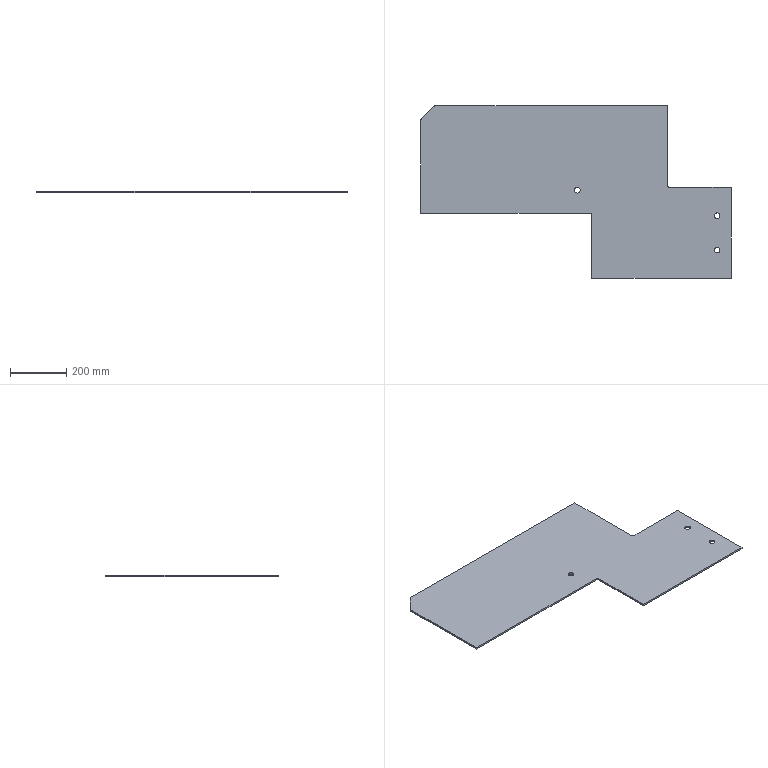Part | SolidWorks | features Fillet 1, FlatPattern 1, SMBaseFlange 1, SheetMetal 1 | 1 solid | 21 faces | box 1100 x 612 x 6 mm | volume 2796793 mm3 | plane 11 | cylinder 10 | commonest cylinder face diameters 20 x8 12 x2
STEP:
#1=CARTESIAN_POINT('',(-555.,312.,-6.));
#2=VERTEX_POINT('',#1);
#3=CARTESIAN_POINT('',(-535.,312.,-6.));
#4=VERTEX_POINT('',#3);
#5=CARTESIAN_POINT('',(-545.,312.,-6.));
#6=DIRECTION('',(0.,0.,1.));
#7=DIRECTION('',(1.,0.,0.));
#8=AXIS2_PLACEMENT_3D('',#5,#6,#7);
#9=CIRCLE('',#8,10.);
#10=EDGE_CURVE('',#2,#4,#9,.T.);
#11=ORIENTED_EDGE('',*,*,#10,.F.);
#12=CARTESIAN_POINT('',(-555.,312.,0.));
#13=VERTEX_POINT('',#12);
#14=CARTESIAN_POINT('',(-555.,312.,-6.));
#15=DIRECTION('',(0.,0.,1.));
#16=VECTOR('',#15,1000.);
#17=LINE('',#14,#16);
#18=EDGE_CURVE('',#2,#13,#17,.T.);
#19=ORIENTED_EDGE('',*,*,#18,.T.);
#20=CARTESIAN_POINT('',(-535.,312.,0.));
#21=VERTEX_POINT('',#20);
#22=CARTESIAN_POINT('',(-545.,312.,0.));
#23=DIRECTION('',(0.,0.,1.));
#24=DIRECTION('',(1.,0.,0.));
#25=AXIS2_PLACEMENT_3D('',#22,#23,#24);
#26=CIRCLE('',#25,10.);
#27=EDGE_CURVE('',#13,#21,#26,.T.);
#28=ORIENTED_EDGE('',*,*,#27,.T.);
#29=CARTESIAN_POINT('',(-535.,312.,-6.));
#30=DIRECTION('',(0.,0.,1.));
#31=VECTOR('',#30,1000.);
#32=LINE('',#29,#31);
#33=EDGE_CURVE('',#4,#21,#32,.T.);
#34=ORIENTED_EDGE('',*,*,#33,.F.);
#35=EDGE_LOOP('',(#11,#19,#28,#34));
#36=FACE_OUTER_BOUND('',#35,.T.);
#37=CARTESIAN_POINT('',(-545.,312.,-6.));
#38=DIRECTION('',(0.,0.,1.));
#39=DIRECTION('',(1.,0.,0.));
#40=AXIS2_PLACEMENT_3D('',#37,#38,#39);
#41=CYLINDRICAL_SURFACE('',#40,10.);
#42=ADVANCED_FACE('',(#36),#41,.F.);
#43=CARTESIAN_POINT('',(-60.,222.,-6.));
#44=VERTEX_POINT('',#43);
#45=CARTESIAN_POINT('',(-40.,222.,-6.));
#46=VERTEX_POINT('',#45);
#47=CARTESIAN_POINT('',(-50.,222.,-6.));
#48=DIRECTION('',(0.,0.,1.));
#49=DIRECTION('',(1.,0.,0.));
#50=AXIS2_PLACEMENT_3D('',#47,#48,#49);
#51=CIRCLE('',#50,10.);
#52=EDGE_CURVE('',#44,#46,#51,.T.);
#53=ORIENTED_EDGE('',*,*,#52,.F.);
#54=CARTESIAN_POINT('',(-60.,222.,0.));
#55=VERTEX_POINT('',#54);
#56=CARTESIAN_POINT('',(-60.,222.,-6.));
#57=DIRECTION('',(0.,0.,1.));
#58=VECTOR('',#57,1000.);
#59=LINE('',#56,#58);
#60=EDGE_CURVE('',#44,#55,#59,.T.);
#61=ORIENTED_EDGE('',*,*,#60,.T.);
#62=CARTESIAN_POINT('',(-40.,222.,0.));
#63=VERTEX_POINT('',#62);
#64=CARTESIAN_POINT('',(-50.,222.,0.));
#65=DIRECTION('',(0.,0.,1.));
#66=DIRECTION('',(1.,0.,0.));
#67=AXIS2_PLACEMENT_3D('',#64,#65,#66);
#68=CIRCLE('',#67,10.);
#69=EDGE_CURVE('',#55,#63,#68,.T.);
#70=ORIENTED_EDGE('',*,*,#69,.T.);
#71=CARTESIAN_POINT('',(-40.,222.,-6.));
#72=DIRECTION('',(0.,0.,1.));
#73=VECTOR('',#72,1000.);
#74=LINE('',#71,#73);
#75=EDGE_CURVE('',#46,#63,#74,.T.);
#76=ORIENTED_EDGE('',*,*,#75,.F.);
#77=EDGE_LOOP('',(#53,#61,#70,#76));
#78=FACE_OUTER_BOUND('',#77,.T.);
#79=CARTESIAN_POINT('',(-50.,222.,-6.));
#80=DIRECTION('',(0.,0.,1.));
#81=DIRECTION('',(1.,0.,0.));
#82=AXIS2_PLACEMENT_3D('',#79,#80,#81);
#83=CYLINDRICAL_SURFACE('',#82,10.);
#84=ADVANCED_FACE('',(#78),#83,.F.);
#85=CARTESIAN_POINT('',(-60.,100.,-6.));
#86=VERTEX_POINT('',#85);
#87=CARTESIAN_POINT('',(-40.,100.,-6.));
#88=VERTEX_POINT('',#87);
#89=CARTESIAN_POINT('',(-50.,100.,-6.));
#90=DIRECTION('',(0.,0.,1.));
#91=DIRECTION('',(1.,0.,0.));
#92=AXIS2_PLACEMENT_3D('',#89,#90,#91);
#93=CIRCLE('',#92,10.);
#94=EDGE_CURVE('',#86,#88,#93,.T.);
#95=ORIENTED_EDGE('',*,*,#94,.F.);
#96=CARTESIAN_POINT('',(-60.,100.,0.));
#97=VERTEX_POINT('',#96);
#98=CARTESIAN_POINT('',(-60.,100.,-6.));
#99=DIRECTION('',(0.,0.,1.));
#100=VECTOR('',#99,1000.);
#101=LINE('',#98,#100);
#102=EDGE_CURVE('',#86,#97,#101,.T.);
#103=ORIENTED_EDGE('',*,*,#102,.T.);
#104=CARTESIAN_POINT('',(-40.,100.,0.));
#105=VERTEX_POINT('',#104);
#106=CARTESIAN_POINT('',(-50.,100.,0.));
#107=DIRECTION('',(0.,0.,1.));
#108=DIRECTION('',(1.,0.,0.));
#109=AXIS2_PLACEMENT_3D('',#106,#107,#108);
#110=CIRCLE('',#109,10.);
#111=EDGE_CURVE('',#97,#105,#110,.T.);
#112=ORIENTED_EDGE('',*,*,#111,.T.);
#113=CARTESIAN_POINT('',(-40.,100.,-6.));
#114=DIRECTION('',(0.,0.,1.));
#115=VECTOR('',#114,1000.);
#116=LINE('',#113,#115);
#117=EDGE_CURVE('',#88,#105,#116,.T.);
#118=ORIENTED_EDGE('',*,*,#117,.F.);
#119=EDGE_LOOP('',(#95,#103,#112,#118));
#120=FACE_OUTER_BOUND('',#119,.T.);
#121=CARTESIAN_POINT('',(-50.,100.,-6.));
#122=DIRECTION('',(0.,0.,1.));
#123=DIRECTION('',(1.,0.,0.));
#124=AXIS2_PLACEMENT_3D('',#121,#122,#123);
#125=CYLINDRICAL_SURFACE('',#124,10.);
#126=ADVANCED_FACE('',(#120),#125,.F.);
#127=CARTESIAN_POINT('',(0.,0.,0.));
#128=VERTEX_POINT('',#127);
#129=CARTESIAN_POINT('',(0.,322.,0.));
#130=VERTEX_POINT('',#129);
#131=CARTESIAN_POINT('',(0.,322.,0.));
#132=DIRECTION('',(0.,1.,0.));
#133=VECTOR('',#132,1000.);
#134=LINE('',#131,#133);
#135=EDGE_CURVE('',#128,#130,#134,.T.);
#136=ORIENTED_EDGE('',*,*,#135,.F.);
#137=CARTESIAN_POINT('',(0.,0.,-6.));
#138=VERTEX_POINT('',#137);
#139=CARTESIAN_POINT('',(0.,0.,-6.));
#140=DIRECTION('',(0.,0.,1.));
#141=VECTOR('',#140,1000.);
#142=LINE('',#139,#141);
#143=EDGE_CURVE('',#138,#128,#142,.T.);
#144=ORIENTED_EDGE('',*,*,#143,.F.);
#145=CARTESIAN_POINT('',(0.,322.,-6.));
#146=VERTEX_POINT('',#145);
#147=CARTESIAN_POINT('',(0.,322.,-6.));
#148=DIRECTION('',(0.,1.,0.));
#149=VECTOR('',#148,1000.);
#150=LINE('',#147,#149);
#151=EDGE_CURVE('',#138,#146,#150,.T.);
#152=ORIENTED_EDGE('',*,*,#151,.T.);
#153=CARTESIAN_POINT('',(0.,322.,-6.));
#154=DIRECTION('',(0.,0.,1.));
#155=VECTOR('',#154,1000.);
#156=LINE('',#153,#155);
#157=EDGE_CURVE('',#146,#130,#156,.T.);
#158=ORIENTED_EDGE('',*,*,#157,.T.);
#159=EDGE_LOOP('',(#136,#144,#152,#158));
#160=FACE_OUTER_BOUND('',#159,.T.);
#161=CARTESIAN_POINT('',(0.,322.,-6.));
#162=DIRECTION('',(1.,0.,0.));
#163=DIRECTION('',(0.,1.,0.));
#164=AXIS2_PLACEMENT_3D('',#161,#162,#163);
#165=PLANE('',#164);
#166=ADVANCED_FACE('',(#160),#165,.T.);
#167=CARTESIAN_POINT('',(-493.5,0.,0.));
#168=VERTEX_POINT('',#167);
#169=CARTESIAN_POINT('',(0.,0.,0.));
#170=DIRECTION('',(1.,0.,0.));
#171=VECTOR('',#170,1000.);
#172=LINE('',#169,#171);
#173=EDGE_CURVE('',#168,#128,#172,.T.);
#174=ORIENTED_EDGE('',*,*,#173,.F.);
#175=CARTESIAN_POINT('',(-493.5,0.,-6.));
#176=VERTEX_POINT('',#175);
#177=CARTESIAN_POINT('',(-493.5,0.,-6.));
#178=DIRECTION('',(0.,0.,1.));
#179=VECTOR('',#178,1000.);
#180=LINE('',#177,#179);
#181=EDGE_CURVE('',#176,#168,#180,.T.);
#182=ORIENTED_EDGE('',*,*,#181,.F.);
#183=CARTESIAN_POINT('',(0.,0.,-6.));
#184=DIRECTION('',(1.,0.,0.));
#185=VECTOR('',#184,1000.);
#186=LINE('',#183,#185);
#187=EDGE_CURVE('',#176,#138,#186,.T.);
#188=ORIENTED_EDGE('',*,*,#187,.T.);
#189=ORIENTED_EDGE('',*,*,#143,.T.);
#190=EDGE_LOOP('',(#174,#182,#188,#189));
#191=FACE_OUTER_BOUND('',#190,.T.);
#192=CARTESIAN_POINT('',(0.,0.,-6.));
#193=DIRECTION('',(0.,-1.,0.));
#194=DIRECTION('',(0.,0.,-1.));
#195=AXIS2_PLACEMENT_3D('',#192,#193,#194);
#196=PLANE('',#195);
#197=ADVANCED_FACE('',(#191),#196,.T.);
#198=CARTESIAN_POINT('',(-493.5,224.,0.));
#199=VERTEX_POINT('',#198);
#200=CARTESIAN_POINT('',(-493.5,0.,0.));
#201=DIRECTION('',(0.,-1.,0.));
#202=VECTOR('',#201,1000.);
#203=LINE('',#200,#202);
#204=EDGE_CURVE('',#199,#168,#203,.T.);
#205=ORIENTED_EDGE('',*,*,#204,.F.);
#206=CARTESIAN_POINT('',(-493.5,224.,-6.));
#207=VERTEX_POINT('',#206);
#208=CARTESIAN_POINT('',(-493.5,224.,-6.));
#209=DIRECTION('',(0.,0.,-1.));
#210=VECTOR('',#209,1000.);
#211=LINE('',#208,#210);
#212=EDGE_CURVE('',#199,#207,#211,.T.);
#213=ORIENTED_EDGE('',*,*,#212,.T.);
#214=CARTESIAN_POINT('',(-493.5,0.,-6.));
#215=DIRECTION('',(0.,-1.,0.));
#216=VECTOR('',#215,1000.);
#217=LINE('',#214,#216);
#218=EDGE_CURVE('',#207,#176,#217,.T.);
#219=ORIENTED_EDGE('',*,*,#218,.T.);
#220=ORIENTED_EDGE('',*,*,#181,.T.);
#221=EDGE_LOOP('',(#205,#213,#219,#220));
#222=FACE_OUTER_BOUND('',#221,.T.);
#223=CARTESIAN_POINT('',(-493.5,0.,-6.));
#224=DIRECTION('',(-1.,0.,0.));
#225=DIRECTION('',(0.,0.,1.));
#226=AXIS2_PLACEMENT_3D('',#223,#224,#225);
#227=PLANE('',#226);
#228=ADVANCED_FACE('',(#222),#227,.T.);
#229=CARTESIAN_POINT('',(-1099.5,230.,-6.));
#230=VERTEX_POINT('',#229);
#231=CARTESIAN_POINT('',(-499.5,230.,-6.));
#232=VERTEX_POINT('',#231);
#233=CARTESIAN_POINT('',(-493.5,230.,-6.));
#234=DIRECTION('',(1.,0.,0.));
#235=VECTOR('',#234,1000.);
#236=LINE('',#233,#235);
#237=EDGE_CURVE('',#230,#232,#236,.T.);
#238=ORIENTED_EDGE('',*,*,#237,.T.);
#239=CARTESIAN_POINT('',(-499.5,230.,0.));
#240=VERTEX_POINT('',#239);
#241=CARTESIAN_POINT('',(-499.5,230.,0.));
#242=DIRECTION('',(0.,0.,1.));
#243=VECTOR('',#242,1000.);
#244=LINE('',#241,#243);
#245=EDGE_CURVE('',#232,#240,#244,.T.);
#246=ORIENTED_EDGE('',*,*,#245,.T.);
#247=CARTESIAN_POINT('',(-1099.5,230.,0.));
#248=VERTEX_POINT('',#247);
#249=CARTESIAN_POINT('',(-493.5,230.,0.));
#250=DIRECTION('',(1.,0.,0.));
#251=VECTOR('',#250,1000.);
#252=LINE('',#249,#251);
#253=EDGE_CURVE('',#248,#240,#252,.T.);
#254=ORIENTED_EDGE('',*,*,#253,.F.);
#255=CARTESIAN_POINT('',(-1099.5,230.,-6.));
#256=DIRECTION('',(0.,0.,1.));
#257=VECTOR('',#256,1000.);
#258=LINE('',#255,#257);
#259=EDGE_CURVE('',#230,#248,#258,.T.);
#260=ORIENTED_EDGE('',*,*,#259,.F.);
#261=EDGE_LOOP('',(#238,#246,#254,#260));
#262=FACE_OUTER_BOUND('',#261,.T.);
#263=CARTESIAN_POINT('',(-493.5,230.,-6.));
#264=DIRECTION('',(0.,-1.,0.));
#265=DIRECTION('',(1.,0.,0.));
#266=AXIS2_PLACEMENT_3D('',#263,#264,#265);
#267=PLANE('',#266);
#268=ADVANCED_FACE('',(#262),#267,.T.);
#269=CARTESIAN_POINT('',(-1099.5,558.858,0.));
#270=VERTEX_POINT('',#269);
#271=CARTESIAN_POINT('',(-1099.5,230.,0.));
#272=DIRECTION('',(0.,-1.,0.));
#273=VECTOR('',#272,1000.);
#274=LINE('',#271,#273);
#275=EDGE_CURVE('',#270,#248,#274,.T.);
#276=ORIENTED_EDGE('',*,*,#275,.F.);
#277=CARTESIAN_POINT('',(-1099.5,558.858,-6.));
#278=VERTEX_POINT('',#277);
#279=CARTESIAN_POINT('',(-1099.5,558.858,-6.));
#280=DIRECTION('',(0.,0.,1.));
#281=VECTOR('',#280,1000.);
#282=LINE('',#279,#281);
#283=EDGE_CURVE('',#278,#270,#282,.T.);
#284=ORIENTED_EDGE('',*,*,#283,.F.);
#285=CARTESIAN_POINT('',(-1099.5,230.,-6.));
#286=DIRECTION('',(0.,-1.,0.));
#287=VECTOR('',#286,1000.);
#288=LINE('',#285,#287);
#289=EDGE_CURVE('',#278,#230,#288,.T.);
#290=ORIENTED_EDGE('',*,*,#289,.T.);
#291=ORIENTED_EDGE('',*,*,#259,.T.);
#292=EDGE_LOOP('',(#276,#284,#290,#291));
#293=FACE_OUTER_BOUND('',#292,.T.);
#294=CARTESIAN_POINT('',(-1099.5,230.,-6.));
#295=DIRECTION('',(-1.,0.,0.));
#296=DIRECTION('',(0.,0.,1.));
#297=AXIS2_PLACEMENT_3D('',#294,#295,#296);
#298=PLANE('',#297);
#299=ADVANCED_FACE('',(#293),#298,.T.);
#300=CARTESIAN_POINT('',(-1096.571,565.929,0.));
#301=VERTEX_POINT('',#300);
#302=CARTESIAN_POINT('',(-1089.5,558.858,0.));
#303=DIRECTION('',(0.,0.,1.));
#304=DIRECTION('',(1.,0.,0.));
#305=AXIS2_PLACEMENT_3D('',#302,#303,#304);
#306=CIRCLE('',#305,10.);
#307=EDGE_CURVE('',#301,#270,#306,.T.);
#308=ORIENTED_EDGE('',*,*,#307,.F.);
#309=CARTESIAN_POINT('',(-1096.571,565.929,-6.));
#310=VERTEX_POINT('',#309);
#311=CARTESIAN_POINT('',(-1096.571,565.929,-6.));
#312=DIRECTION('',(0.,0.,1.));
#313=VECTOR('',#312,1000.);
#314=LINE('',#311,#313);
#315=EDGE_CURVE('',#310,#301,#314,.T.);
#316=ORIENTED_EDGE('',*,*,#315,.F.);
#317=CARTESIAN_POINT('',(-1089.5,558.858,-6.));
#318=DIRECTION('',(0.,0.,1.));
#319=DIRECTION('',(1.,0.,0.));
#320=AXIS2_PLACEMENT_3D('',#317,#318,#319);
#321=CIRCLE('',#320,10.);
#322=EDGE_CURVE('',#310,#278,#321,.T.);
#323=ORIENTED_EDGE('',*,*,#322,.T.);
#324=ORIENTED_EDGE('',*,*,#283,.T.);
#325=EDGE_LOOP('',(#308,#316,#323,#324));
#326=FACE_OUTER_BOUND('',#325,.T.);
#327=CARTESIAN_POINT('',(-1089.5,558.858,-6.));
#328=DIRECTION('',(0.,0.,1.));
#329=DIRECTION('',(1.,0.,0.));
#330=AXIS2_PLACEMENT_3D('',#327,#328,#329);
#331=CYLINDRICAL_SURFACE('',#330,10.);
#332=ADVANCED_FACE('',(#326),#331,.T.);
#333=CARTESIAN_POINT('',(-1053.429,609.071,0.));
#334=VERTEX_POINT('',#333);
#335=CARTESIAN_POINT('',(-1096.571,565.929,0.));
#336=DIRECTION('',(-0.7071,-0.7071,0.));
#337=VECTOR('',#336,1000.);
#338=LINE('',#335,#337);
#339=EDGE_CURVE('',#334,#301,#338,.T.);
#340=ORIENTED_EDGE('',*,*,#339,.F.);
#341=CARTESIAN_POINT('',(-1053.429,609.071,-6.));
#342=VERTEX_POINT('',#341);
#343=CARTESIAN_POINT('',(-1053.429,609.071,-6.));
#344=DIRECTION('',(0.,0.,1.));
#345=VECTOR('',#344,1000.);
#346=LINE('',#343,#345);
#347=EDGE_CURVE('',#342,#334,#346,.T.);
#348=ORIENTED_EDGE('',*,*,#347,.F.);
#349=CARTESIAN_POINT('',(-1096.571,565.929,-6.));
#350=DIRECTION('',(-0.7071,-0.7071,0.));
#351=VECTOR('',#350,1000.);
#352=LINE('',#349,#351);
#353=EDGE_CURVE('',#342,#310,#352,.T.);
#354=ORIENTED_EDGE('',*,*,#353,.T.);
#355=ORIENTED_EDGE('',*,*,#315,.T.);
#356=EDGE_LOOP('',(#340,#348,#354,#355));
#357=FACE_OUTER_BOUND('',#356,.T.);
#358=CARTESIAN_POINT('',(-1096.571,565.929,-6.));
#359=DIRECTION('',(-0.7071,0.7071,0.));
#360=DIRECTION('',(-0.7071,-0.7071,0.));
#361=AXIS2_PLACEMENT_3D('',#358,#359,#360);
#362=PLANE('',#361);
#363=ADVANCED_FACE('',(#357),#362,.T.);
#364=CARTESIAN_POINT('',(-1046.358,612.,0.));
#365=VERTEX_POINT('',#364);
#366=CARTESIAN_POINT('',(-1046.358,602.,0.));
#367=DIRECTION('',(0.,0.,1.));
#368=DIRECTION('',(-1.,0.,0.));
#369=AXIS2_PLACEMENT_3D('',#366,#367,#368);
#370=CIRCLE('',#369,10.);
#371=EDGE_CURVE('',#365,#334,#370,.T.);
#372=ORIENTED_EDGE('',*,*,#371,.F.);
#373=CARTESIAN_POINT('',(-1046.358,612.,-6.));
#374=VERTEX_POINT('',#373);
#375=CARTESIAN_POINT('',(-1046.358,612.,-6.));
#376=DIRECTION('',(0.,0.,1.));
#377=VECTOR('',#376,1000.);
#378=LINE('',#375,#377);
#379=EDGE_CURVE('',#374,#365,#378,.T.);
#380=ORIENTED_EDGE('',*,*,#379,.F.);
#381=CARTESIAN_POINT('',(-1046.358,602.,-6.));
#382=DIRECTION('',(0.,0.,1.));
#383=DIRECTION('',(-1.,0.,0.));
#384=AXIS2_PLACEMENT_3D('',#381,#382,#383);
#385=CIRCLE('',#384,10.);
#386=EDGE_CURVE('',#374,#342,#385,.T.);
#387=ORIENTED_EDGE('',*,*,#386,.T.);
#388=ORIENTED_EDGE('',*,*,#347,.T.);
#389=EDGE_LOOP('',(#372,#380,#387,#388));
#390=FACE_OUTER_BOUND('',#389,.T.);
#391=CARTESIAN_POINT('',(-1046.358,602.,-6.));
#392=DIRECTION('',(0.,0.,1.));
#393=DIRECTION('',(1.,0.,0.));
#394=AXIS2_PLACEMENT_3D('',#391,#392,#393);
#395=CYLINDRICAL_SURFACE('',#394,10.);
#396=ADVANCED_FACE('',(#390),#395,.T.);
#397=CARTESIAN_POINT('',(-225.,612.,0.));
#398=VERTEX_POINT('',#397);
#399=CARTESIAN_POINT('',(-1046.358,612.,0.));
#400=DIRECTION('',(-1.,0.,0.));
#401=VECTOR('',#400,1000.);
#402=LINE('',#399,#401);
#403=EDGE_CURVE('',#398,#365,#402,.T.);
#404=ORIENTED_EDGE('',*,*,#403,.F.);
#405=CARTESIAN_POINT('',(-225.,612.,-6.));
#406=VERTEX_POINT('',#405);
#407=CARTESIAN_POINT('',(-225.,612.,-6.));
#408=DIRECTION('',(0.,0.,1.));
#409=VECTOR('',#408,1000.);
#410=LINE('',#407,#409);
#411=EDGE_CURVE('',#406,#398,#410,.T.);
#412=ORIENTED_EDGE('',*,*,#411,.F.);
#413=CARTESIAN_POINT('',(-1046.358,612.,-6.));
#414=DIRECTION('',(-1.,0.,0.));
#415=VECTOR('',#414,1000.);
#416=LINE('',#413,#415);
#417=EDGE_CURVE('',#406,#374,#416,.T.);
#418=ORIENTED_EDGE('',*,*,#417,.T.);
#419=ORIENTED_EDGE('',*,*,#379,.T.);
#420=EDGE_LOOP('',(#404,#412,#418,#419));
#421=FACE_OUTER_BOUND('',#420,.T.);
#422=CARTESIAN_POINT('',(-1046.358,612.,-6.));
#423=DIRECTION('',(0.,1.,0.));
#424=DIRECTION('',(0.,0.,1.));
#425=AXIS2_PLACEMENT_3D('',#422,#423,#424);
#426=PLANE('',#425);
#427=ADVANCED_FACE('',(#421),#426,.T.);
#428=CARTESIAN_POINT('',(-225.,328.,0.));
#429=VERTEX_POINT('',#428);
#430=CARTESIAN_POINT('',(-225.,612.,0.));
#431=DIRECTION('',(0.,1.,0.));
#432=VECTOR('',#431,1000.);
#433=LINE('',#430,#432);
#434=EDGE_CURVE('',#429,#398,#433,.T.);
#435=ORIENTED_EDGE('',*,*,#434,.F.);
#436=CARTESIAN_POINT('',(-225.,328.,-6.));
#437=VERTEX_POINT('',#436);
#438=CARTESIAN_POINT('',(-225.,328.,-6.));
#439=DIRECTION('',(0.,0.,-1.));
#440=VECTOR('',#439,1000.);
#441=LINE('',#438,#440);
#442=EDGE_CURVE('',#429,#437,#441,.T.);
#443=ORIENTED_EDGE('',*,*,#442,.T.);
#444=CARTESIAN_POINT('',(-225.,612.,-6.));
#445=DIRECTION('',(0.,1.,0.));
#446=VECTOR('',#445,1000.);
#447=LINE('',#444,#446);
#448=EDGE_CURVE('',#437,#406,#447,.T.);
#449=ORIENTED_EDGE('',*,*,#448,.T.);
#450=ORIENTED_EDGE('',*,*,#411,.T.);
#451=EDGE_LOOP('',(#435,#443,#449,#450));
#452=FACE_OUTER_BOUND('',#451,.T.);
#453=CARTESIAN_POINT('',(-225.,612.,-6.));
#454=DIRECTION('',(1.,0.,0.));
#455=DIRECTION('',(0.,1.,0.));
#456=AXIS2_PLACEMENT_3D('',#453,#454,#455);
#457=PLANE('',#456);
#458=ADVANCED_FACE('',(#452),#457,.T.);
#459=CARTESIAN_POINT('',(-219.,322.,-6.));
#460=VERTEX_POINT('',#459);
#461=CARTESIAN_POINT('',(-225.,322.,-6.));
#462=DIRECTION('',(-1.,0.,0.));
#463=VECTOR('',#462,1000.);
#464=LINE('',#461,#463);
#465=EDGE_CURVE('',#146,#460,#464,.T.);
#466=ORIENTED_EDGE('',*,*,#465,.T.);
#467=CARTESIAN_POINT('',(-219.,322.,0.));
#468=VERTEX_POINT('',#467);
#469=CARTESIAN_POINT('',(-219.,322.,0.));
#470=DIRECTION('',(0.,0.,1.));
#471=VECTOR('',#470,1000.);
#472=LINE('',#469,#471);
#473=EDGE_CURVE('',#460,#468,#472,.T.);
#474=ORIENTED_EDGE('',*,*,#473,.T.);
#475=CARTESIAN_POINT('',(-225.,322.,0.));
#476=DIRECTION('',(-1.,0.,0.));
#477=VECTOR('',#476,1000.);
#478=LINE('',#475,#477);
#479=EDGE_CURVE('',#130,#468,#478,.T.);
#480=ORIENTED_EDGE('',*,*,#479,.F.);
#481=ORIENTED_EDGE('',*,*,#157,.F.);
#482=EDGE_LOOP('',(#466,#474,#480,#481));
#483=FACE_OUTER_BOUND('',#482,.T.);
#484=CARTESIAN_POINT('',(-225.,322.,-6.));
#485=DIRECTION('',(0.,1.,0.));
#486=DIRECTION('',(0.,0.,1.));
#487=AXIS2_PLACEMENT_3D('',#484,#485,#486);
#488=PLANE('',#487);
#489=ADVANCED_FACE('',(#483),#488,.T.);
#490=CARTESIAN_POINT('',(-545.,312.,-6.));
#491=DIRECTION('',(0.,0.,1.));
#492=DIRECTION('',(1.,0.,0.));
#493=AXIS2_PLACEMENT_3D('',#490,#491,#492);
#494=CIRCLE('',#493,10.);
#495=EDGE_CURVE('',#4,#2,#494,.T.);
#496=ORIENTED_EDGE('',*,*,#495,.T.);
#497=ORIENTED_EDGE('',*,*,#10,.T.);
#498=EDGE_LOOP('',(#496,#497));
#499=FACE_BOUND('',#498,.T.);
#500=CARTESIAN_POINT('',(-50.,222.,-6.));
#501=DIRECTION('',(0.,0.,1.));
#502=DIRECTION('',(1.,0.,0.));
#503=AXIS2_PLACEMENT_3D('',#500,#501,#502);
#504=CIRCLE('',#503,10.);
#505=EDGE_CURVE('',#46,#44,#504,.T.);
#506=ORIENTED_EDGE('',*,*,#505,.T.);
#507=ORIENTED_EDGE('',*,*,#52,.T.);
#508=EDGE_LOOP('',(#506,#507));
#509=FACE_BOUND('',#508,.T.);
#510=CARTESIAN_POINT('',(-50.,100.,-6.));
#511=DIRECTION('',(0.,0.,1.));
#512=DIRECTION('',(1.,0.,0.));
#513=AXIS2_PLACEMENT_3D('',#510,#511,#512);
#514=CIRCLE('',#513,10.);
#515=EDGE_CURVE('',#88,#86,#514,.T.);
#516=ORIENTED_EDGE('',*,*,#515,.T.);
#517=ORIENTED_EDGE('',*,*,#94,.T.);
#518=EDGE_LOOP('',(#516,#517));
#519=FACE_BOUND('',#518,.T.);
#520=ORIENTED_EDGE('',*,*,#151,.F.);
#521=ORIENTED_EDGE('',*,*,#187,.F.);
#522=ORIENTED_EDGE('',*,*,#218,.F.);
#523=CARTESIAN_POINT('',(-499.5,224.,-6.));
#524=DIRECTION('',(0.,0.,1.));
#525=DIRECTION('',(1.,0.,0.));
#526=AXIS2_PLACEMENT_3D('',#523,#524,#525);
#527=CIRCLE('',#526,6.);
#528=EDGE_CURVE('',#207,#232,#527,.T.);
#529=ORIENTED_EDGE('',*,*,#528,.T.);
#530=ORIENTED_EDGE('',*,*,#237,.F.);
#531=ORIENTED_EDGE('',*,*,#289,.F.);
#532=ORIENTED_EDGE('',*,*,#322,.F.);
#533=ORIENTED_EDGE('',*,*,#353,.F.);
#534=ORIENTED_EDGE('',*,*,#386,.F.);
#535=ORIENTED_EDGE('',*,*,#417,.F.);
#536=ORIENTED_EDGE('',*,*,#448,.F.);
#537=CARTESIAN_POINT('',(-219.,328.,-6.));
#538=DIRECTION('',(0.,0.,1.));
#539=DIRECTION('',(1.,0.,0.));
#540=AXIS2_PLACEMENT_3D('',#537,#538,#539);
#541=CIRCLE('',#540,6.);
#542=EDGE_CURVE('',#437,#460,#541,.T.);
#543=ORIENTED_EDGE('',*,*,#542,.T.);
#544=ORIENTED_EDGE('',*,*,#465,.F.);
#545=EDGE_LOOP('',(#520,#521,#522,#529,#530,#531,#532,#533,#534,#535,#536,#543,#544));
#546=FACE_OUTER_BOUND('',#545,.T.);
#547=CARTESIAN_POINT('',(-1089.5,558.858,-6.));
#548=DIRECTION('',(0.,0.,1.));
#549=DIRECTION('',(1.,0.,0.));
#550=AXIS2_PLACEMENT_3D('',#547,#548,#549);
#551=PLANE('',#550);
#552=ADVANCED_FACE('',(#499,#509,#519,#546),#551,.F.);
#553=CARTESIAN_POINT('',(-545.,312.,0.));
#554=DIRECTION('',(0.,0.,1.));
#555=DIRECTION('',(1.,0.,0.));
#556=AXIS2_PLACEMENT_3D('',#553,#554,#555);
#557=CIRCLE('',#556,10.);
#558=EDGE_CURVE('',#21,#13,#557,.T.);
#559=ORIENTED_EDGE('',*,*,#558,.F.);
#560=ORIENTED_EDGE('',*,*,#27,.F.);
#561=EDGE_LOOP('',(#559,#560));
#562=FACE_BOUND('',#561,.T.);
#563=CARTESIAN_POINT('',(-50.,222.,0.));
#564=DIRECTION('',(0.,0.,1.));
#565=DIRECTION('',(1.,0.,0.));
#566=AXIS2_PLACEMENT_3D('',#563,#564,#565);
#567=CIRCLE('',#566,10.);
#568=EDGE_CURVE('',#63,#55,#567,.T.);
#569=ORIENTED_EDGE('',*,*,#568,.F.);
#570=ORIENTED_EDGE('',*,*,#69,.F.);
#571=EDGE_LOOP('',(#569,#570));
#572=FACE_BOUND('',#571,.T.);
#573=CARTESIAN_POINT('',(-50.,100.,0.));
#574=DIRECTION('',(0.,0.,1.));
#575=DIRECTION('',(1.,0.,0.));
#576=AXIS2_PLACEMENT_3D('',#573,#574,#575);
#577=CIRCLE('',#576,10.);
#578=EDGE_CURVE('',#105,#97,#577,.T.);
#579=ORIENTED_EDGE('',*,*,#578,.F.);
#580=ORIENTED_EDGE('',*,*,#111,.F.);
#581=EDGE_LOOP('',(#579,#580));
#582=FACE_BOUND('',#581,.T.);
#583=ORIENTED_EDGE('',*,*,#135,.T.);
#584=ORIENTED_EDGE('',*,*,#479,.T.);
#585=CARTESIAN_POINT('',(-219.,328.,0.));
#586=DIRECTION('',(0.,0.,-1.));
#587=DIRECTION('',(1.,0.,0.));
#588=AXIS2_PLACEMENT_3D('',#585,#586,#587);
#589=CIRCLE('',#588,6.);
#590=EDGE_CURVE('',#468,#429,#589,.T.);
#591=ORIENTED_EDGE('',*,*,#590,.T.);
#592=ORIENTED_EDGE('',*,*,#434,.T.);
#593=ORIENTED_EDGE('',*,*,#403,.T.);
#594=ORIENTED_EDGE('',*,*,#371,.T.);
#595=ORIENTED_EDGE('',*,*,#339,.T.);
#596=ORIENTED_EDGE('',*,*,#307,.T.);
#597=ORIENTED_EDGE('',*,*,#275,.T.);
#598=ORIENTED_EDGE('',*,*,#253,.T.);
#599=CARTESIAN_POINT('',(-499.5,224.,0.));
#600=DIRECTION('',(0.,0.,-1.));
#601=DIRECTION('',(1.,0.,0.));
#602=AXIS2_PLACEMENT_3D('',#599,#600,#601);
#603=CIRCLE('',#602,6.);
#604=EDGE_CURVE('',#240,#199,#603,.T.);
#605=ORIENTED_EDGE('',*,*,#604,.T.);
#606=ORIENTED_EDGE('',*,*,#204,.T.);
#607=ORIENTED_EDGE('',*,*,#173,.T.);
#608=EDGE_LOOP('',(#583,#584,#591,#592,#593,#594,#595,#596,#597,#598,#605,#606,#607));
#609=FACE_OUTER_BOUND('',#608,.T.);
#610=CARTESIAN_POINT('',(-1089.5,558.858,0.));
#611=DIRECTION('',(0.,0.,1.));
#612=DIRECTION('',(1.,0.,0.));
#613=AXIS2_PLACEMENT_3D('',#610,#611,#612);
#614=PLANE('',#613);
#615=ADVANCED_FACE('',(#562,#572,#582,#609),#614,.T.);
#616=ORIENTED_EDGE('',*,*,#102,.F.);
#617=ORIENTED_EDGE('',*,*,#515,.F.);
#618=ORIENTED_EDGE('',*,*,#117,.T.);
#619=ORIENTED_EDGE('',*,*,#578,.T.);
#620=EDGE_LOOP('',(#616,#617,#618,#619));
#621=FACE_OUTER_BOUND('',#620,.T.);
#622=CARTESIAN_POINT('',(-50.,100.,-6.));
#623=DIRECTION('',(0.,0.,1.));
#624=DIRECTION('',(1.,0.,0.));
#625=AXIS2_PLACEMENT_3D('',#622,#623,#624);
#626=CYLINDRICAL_SURFACE('',#625,10.);
#627=ADVANCED_FACE('',(#621),#626,.F.);
#628=ORIENTED_EDGE('',*,*,#60,.F.);
#629=ORIENTED_EDGE('',*,*,#505,.F.);
#630=ORIENTED_EDGE('',*,*,#75,.T.);
#631=ORIENTED_EDGE('',*,*,#568,.T.);
#632=EDGE_LOOP('',(#628,#629,#630,#631));
#633=FACE_OUTER_BOUND('',#632,.T.);
#634=CARTESIAN_POINT('',(-50.,222.,-6.));
#635=DIRECTION('',(0.,0.,1.));
#636=DIRECTION('',(1.,0.,0.));
#637=AXIS2_PLACEMENT_3D('',#634,#635,#636);
#638=CYLINDRICAL_SURFACE('',#637,10.);
#639=ADVANCED_FACE('',(#633),#638,.F.);
#640=ORIENTED_EDGE('',*,*,#18,.F.);
#641=ORIENTED_EDGE('',*,*,#495,.F.);
#642=ORIENTED_EDGE('',*,*,#33,.T.);
#643=ORIENTED_EDGE('',*,*,#558,.T.);
#644=EDGE_LOOP('',(#640,#641,#642,#643));
#645=FACE_OUTER_BOUND('',#644,.T.);
#646=CARTESIAN_POINT('',(-545.,312.,-6.));
#647=DIRECTION('',(0.,0.,1.));
#648=DIRECTION('',(1.,0.,0.));
#649=AXIS2_PLACEMENT_3D('',#646,#647,#648);
#650=CYLINDRICAL_SURFACE('',#649,10.);
#651=ADVANCED_FACE('',(#645),#650,.F.);
#652=ORIENTED_EDGE('',*,*,#528,.F.);
#653=ORIENTED_EDGE('',*,*,#212,.F.);
#654=ORIENTED_EDGE('',*,*,#604,.F.);
#655=ORIENTED_EDGE('',*,*,#245,.F.);
#656=EDGE_LOOP('',(#652,#653,#654,#655));
#657=FACE_OUTER_BOUND('',#656,.T.);
#658=CARTESIAN_POINT('',(-499.5,224.,-6.));
#659=DIRECTION('',(0.,0.,-1.));
#660=DIRECTION('',(-1.,0.,0.));
#661=AXIS2_PLACEMENT_3D('',#658,#659,#660);
#662=CYLINDRICAL_SURFACE('',#661,6.);
#663=ADVANCED_FACE('',(#657),#662,.F.);
#664=ORIENTED_EDGE('',*,*,#542,.F.);
#665=ORIENTED_EDGE('',*,*,#442,.F.);
#666=ORIENTED_EDGE('',*,*,#590,.F.);
#667=ORIENTED_EDGE('',*,*,#473,.F.);
#668=EDGE_LOOP('',(#664,#665,#666,#667));
#669=FACE_OUTER_BOUND('',#668,.T.);
#670=CARTESIAN_POINT('',(-219.,328.,-6.));
#671=DIRECTION('',(0.,0.,-1.));
#672=DIRECTION('',(-1.,0.,0.));
#673=AXIS2_PLACEMENT_3D('',#670,#671,#672);
#674=CYLINDRICAL_SURFACE('',#673,6.);
#675=ADVANCED_FACE('',(#669),#674,.F.);
#676=CLOSED_SHELL('',(#42,#84,#126,#166,#197,#228,#268,#299,#332,#363,#396,#427,#458,#489,#552,#615,#627,#639,#651,#663,#675));
#677=MANIFOLD_SOLID_BREP('',#676);
#678=CARTESIAN_POINT('',(0.,0.,0.));
#679=DIRECTION('',(0.,0.,1.));
#680=DIRECTION('',(1.,0.,0.));
#681=AXIS2_PLACEMENT_3D('',#678,#679,#680);
#682=(LENGTH_UNIT()NAMED_UNIT(*)SI_UNIT(.MILLI.,.METRE.));
#683=UNCERTAINTY_MEASURE_WITH_UNIT(LENGTH_MEASURE(0.00001),#682,'','');
#684=(NAMED_UNIT(*)PLANE_ANGLE_UNIT()SI_UNIT($,.RADIAN.));
#685=(NAMED_UNIT(*)SI_UNIT($,.STERADIAN.)SOLID_ANGLE_UNIT());
#686=(GEOMETRIC_REPRESENTATION_CONTEXT(3)GLOBAL_UNCERTAINTY_ASSIGNED_CONTEXT((#683))GLOBAL_UNIT_ASSIGNED_CONTEXT((#682,#684,#685))REPRESENTATION_CONTEXT('',''));
#687=ADVANCED_BREP_SHAPE_REPRESENTATION('',(#677,#681),#686);